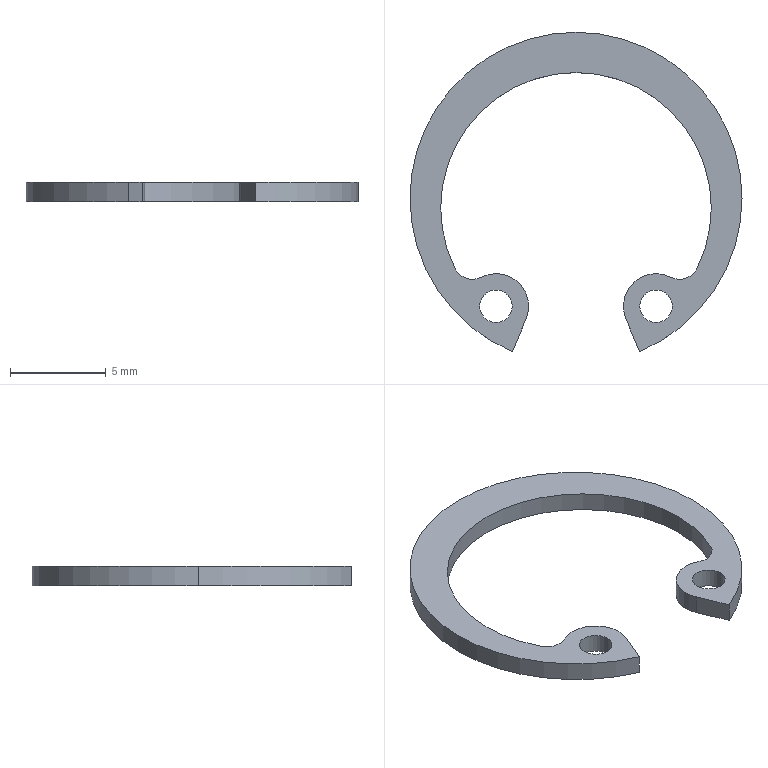Part | STEP file | circlips for holes--type a gb_GB_CONNECTING_PIECE_RING_RRH 16 | 1 solid | 19 faces | box 17.3 x 16.642 x 1 mm | volume 79.55 mm3 | cylinder 15 | plane 4 | commonest cylinder face diameters 1.7 x4 3.4 x3 14.1 x3 17.3 x3 2 x2